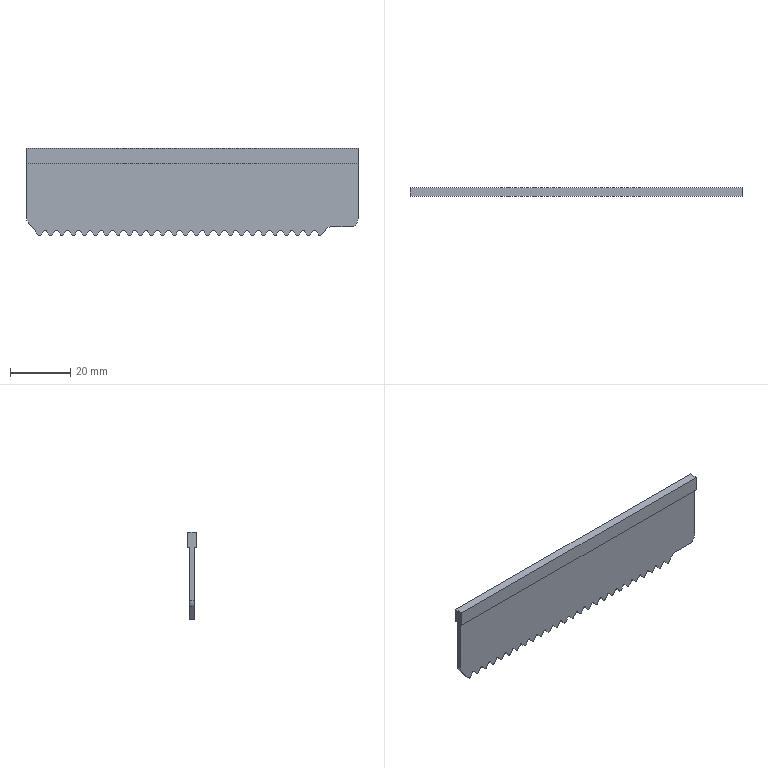Part | STEP file | 200 mesh_id1902 | 1 solid | 117 faces | box 109.8 x 2.8 x 28.9 mm | volume 4981 mm3 | plane 63 | cylinder 54 | commonest cylinder face diameters 0.84 x26 0.8 x25 6 x2 4 x1